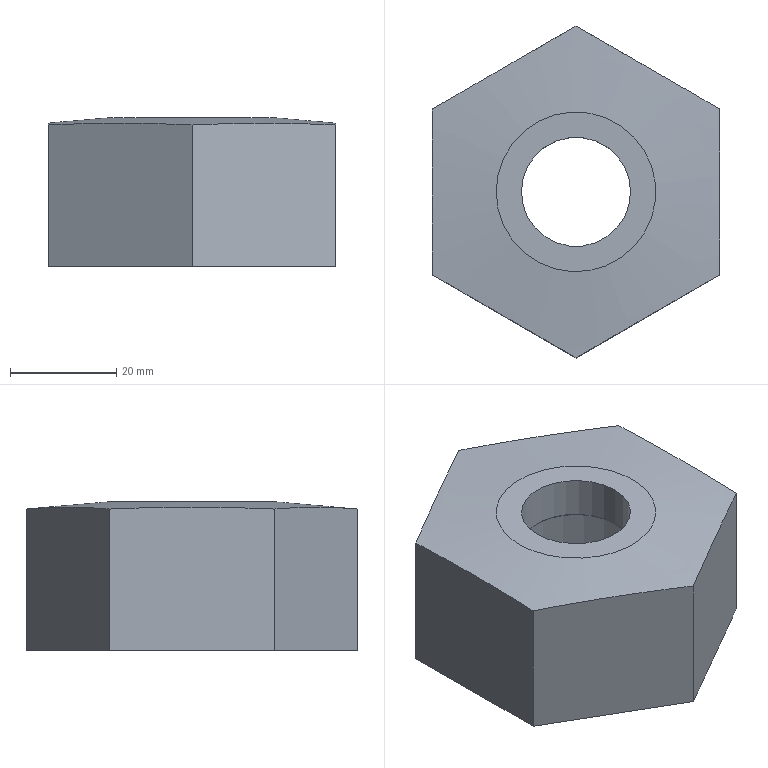Part | NX | features DATUM_CSYS 3, CYLINDER 2, SKETCH 2, CHAMFER 1, EXTRUDE 1, HOLE PACKAGE 1, SIMPLE HOLE 1, SWP104 1, SYMBOLIC_THREAD 1 | 1 solid | 16 faces | box 54.002 x 62.354 x 28 mm | volume 36749 mm3 | plane 10 | cylinder 3 | cone 3 | commonest cylinder face diameters 20.5 x1 43.5 x1 46 x1
STEP:
#1=CARTESIAN_POINT('',(10.25,0.,28.));
#2=VERTEX_POINT('',#1);
#3=CARTESIAN_POINT('',(0.,0.,28.));
#4=DIRECTION('',(0.,0.,1.));
#5=DIRECTION('',(1.,0.,0.));
#6=AXIS2_PLACEMENT_3D('',#3,#4,#5);
#7=CIRCLE('',#6,10.25);
#8=EDGE_CURVE('',#2,#2,#7,.T.);
#9=ORIENTED_EDGE('',*,*,#8,.F.);
#10=EDGE_LOOP('',(#9));
#11=FACE_BOUND('',#10,.T.);
#12=CARTESIAN_POINT('',(-15.,0.,28.));
#13=VERTEX_POINT('',#12);
#14=CARTESIAN_POINT('',(0.,0.,28.));
#15=DIRECTION('',(0.,0.,-1.));
#16=DIRECTION('',(-1.,0.,0.));
#17=AXIS2_PLACEMENT_3D('',#14,#15,#16);
#18=CIRCLE('',#17,15.);
#19=EDGE_CURVE('',#13,#13,#18,.T.);
#20=ORIENTED_EDGE('',*,*,#19,.F.);
#21=EDGE_LOOP('',(#20));
#22=FACE_BOUND('',#21,.T.);
#23=CARTESIAN_POINT('',(0.,0.,28.));
#24=DIRECTION('',(0.,0.,1.));
#25=DIRECTION('',(1.,0.,0.));
#26=AXIS2_PLACEMENT_3D('',#23,#24,#25);
#27=PLANE('',#26);
#28=ADVANCED_FACE('',(#11,#22),#27,.T.);
#29=CARTESIAN_POINT('',(-27.,-15.588,26.585));
#30=VERTEX_POINT('',#29);
#31=CARTESIAN_POINT('',(-27.,-15.588,0.));
#32=VERTEX_POINT('',#31);
#33=CARTESIAN_POINT('',(-27.,-15.588,28.));
#34=DIRECTION('',(0.,0.,-1.));
#35=VECTOR('',#34,1000.);
#36=LINE('',#33,#35);
#37=EDGE_CURVE('',#30,#32,#36,.T.);
#38=ORIENTED_EDGE('',*,*,#37,.F.);
#39=CARTESIAN_POINT('',(-27.,15.588,26.585));
#40=VERTEX_POINT('',#39);
#41=CARTESIAN_POINT('',(-27.,-15.588,26.585));
#42=CARTESIAN_POINT('',(-27.,-5.198,27.039));
#43=CARTESIAN_POINT('',(-27.,5.2,27.039));
#44=CARTESIAN_POINT('',(-27.,15.588,26.585));
#45=B_SPLINE_CURVE_WITH_KNOTS('',3,(#41,#42,#43,#44),.UNSPECIFIED.,.F.,.F.,(4,4),(0.02557,0.05677),.UNSPECIFIED.);
#46=EDGE_CURVE('',#30,#40,#45,.T.);
#47=ORIENTED_EDGE('',*,*,#46,.T.);
#48=CARTESIAN_POINT('',(-27.,15.588,0.));
#49=VERTEX_POINT('',#48);
#50=CARTESIAN_POINT('',(-27.,15.588,28.));
#51=DIRECTION('',(0.,0.,-1.));
#52=VECTOR('',#51,1000.);
#53=LINE('',#50,#52);
#54=EDGE_CURVE('',#40,#49,#53,.T.);
#55=ORIENTED_EDGE('',*,*,#54,.T.);
#56=CARTESIAN_POINT('',(-27.,15.588,0.));
#57=DIRECTION('',(0.,-1.,0.));
#58=VECTOR('',#57,1000.);
#59=LINE('',#56,#58);
#60=EDGE_CURVE('',#49,#32,#59,.T.);
#61=ORIENTED_EDGE('',*,*,#60,.T.);
#62=EDGE_LOOP('',(#38,#47,#55,#61));
#63=FACE_BOUND('',#62,.T.);
#64=CARTESIAN_POINT('',(-27.,15.588,28.));
#65=DIRECTION('',(1.,0.,0.));
#66=DIRECTION('',(0.,0.,-1.));
#67=AXIS2_PLACEMENT_3D('',#64,#65,#66);
#68=PLANE('',#67);
#69=ADVANCED_FACE('',(#63),#68,.F.);
#70=CARTESIAN_POINT('',(0.,-31.177,26.585));
#71=VERTEX_POINT('',#70);
#72=CARTESIAN_POINT('',(0.,-31.177,0.));
#73=VERTEX_POINT('',#72);
#74=CARTESIAN_POINT('',(0.,-31.177,28.));
#75=DIRECTION('',(0.,0.,-1.));
#76=VECTOR('',#75,1000.);
#77=LINE('',#74,#76);
#78=EDGE_CURVE('',#71,#73,#77,.T.);
#79=ORIENTED_EDGE('',*,*,#78,.F.);
#80=CARTESIAN_POINT('',(0.,-31.177,26.585));
#81=CARTESIAN_POINT('',(-9.,-25.981,27.039));
#82=CARTESIAN_POINT('',(-18.,-20.785,27.039));
#83=CARTESIAN_POINT('',(-27.,-15.588,26.585));
#84=B_SPLINE_CURVE_WITH_KNOTS('',3,(#80,#81,#82,#83),.UNSPECIFIED.,.F.,.F.,(4,4),(0.000000231,0.03118),.UNSPECIFIED.);
#85=EDGE_CURVE('',#71,#30,#84,.T.);
#86=ORIENTED_EDGE('',*,*,#85,.T.);
#87=ORIENTED_EDGE('',*,*,#37,.T.);
#88=CARTESIAN_POINT('',(-27.,-15.588,0.));
#89=DIRECTION('',(0.866,-0.5,0.));
#90=VECTOR('',#89,1000.);
#91=LINE('',#88,#90);
#92=EDGE_CURVE('',#32,#73,#91,.T.);
#93=ORIENTED_EDGE('',*,*,#92,.T.);
#94=EDGE_LOOP('',(#79,#86,#87,#93));
#95=FACE_BOUND('',#94,.T.);
#96=CARTESIAN_POINT('',(-27.,-15.588,28.));
#97=DIRECTION('',(0.5,0.866,0.));
#98=DIRECTION('',(-0.866,0.5,0.));
#99=AXIS2_PLACEMENT_3D('',#96,#97,#98);
#100=PLANE('',#99);
#101=ADVANCED_FACE('',(#95),#100,.F.);
#102=CARTESIAN_POINT('',(27.,-15.588,26.585));
#103=VERTEX_POINT('',#102);
#104=CARTESIAN_POINT('',(27.,-15.588,0.));
#105=VERTEX_POINT('',#104);
#106=CARTESIAN_POINT('',(27.,-15.588,28.));
#107=DIRECTION('',(0.,0.,-1.));
#108=VECTOR('',#107,1000.);
#109=LINE('',#106,#108);
#110=EDGE_CURVE('',#103,#105,#109,.T.);
#111=ORIENTED_EDGE('',*,*,#110,.F.);
#112=CARTESIAN_POINT('',(27.,-15.588,26.585));
#113=CARTESIAN_POINT('',(18.,-20.785,27.039));
#114=CARTESIAN_POINT('',(9.,-25.981,27.039));
#115=CARTESIAN_POINT('',(0.,-31.177,26.585));
#116=B_SPLINE_CURVE_WITH_KNOTS('',3,(#112,#113,#114,#115),.UNSPECIFIED.,.F.,.F.,(4,4),(0.000000231,0.03118),.UNSPECIFIED.);
#117=EDGE_CURVE('',#103,#71,#116,.T.);
#118=ORIENTED_EDGE('',*,*,#117,.T.);
#119=ORIENTED_EDGE('',*,*,#78,.T.);
#120=CARTESIAN_POINT('',(0.,-31.177,0.));
#121=DIRECTION('',(0.866,0.5,0.));
#122=VECTOR('',#121,1000.);
#123=LINE('',#120,#122);
#124=EDGE_CURVE('',#73,#105,#123,.T.);
#125=ORIENTED_EDGE('',*,*,#124,.T.);
#126=EDGE_LOOP('',(#111,#118,#119,#125));
#127=FACE_BOUND('',#126,.T.);
#128=CARTESIAN_POINT('',(0.,-31.177,28.));
#129=DIRECTION('',(-0.5,0.866,0.));
#130=DIRECTION('',(-0.866,-0.5,0.));
#131=AXIS2_PLACEMENT_3D('',#128,#129,#130);
#132=PLANE('',#131);
#133=ADVANCED_FACE('',(#127),#132,.F.);
#134=CARTESIAN_POINT('',(27.,15.588,26.585));
#135=VERTEX_POINT('',#134);
#136=CARTESIAN_POINT('',(27.,15.588,0.));
#137=VERTEX_POINT('',#136);
#138=CARTESIAN_POINT('',(27.,15.588,28.));
#139=DIRECTION('',(0.,0.,-1.));
#140=VECTOR('',#139,1000.);
#141=LINE('',#138,#140);
#142=EDGE_CURVE('',#135,#137,#141,.T.);
#143=ORIENTED_EDGE('',*,*,#142,.F.);
#144=CARTESIAN_POINT('',(27.,-15.588,26.585));
#145=CARTESIAN_POINT('',(27.,-5.198,27.039));
#146=CARTESIAN_POINT('',(27.,5.2,27.039));
#147=CARTESIAN_POINT('',(27.,15.588,26.585));
#148=B_SPLINE_CURVE_WITH_KNOTS('',3,(#144,#145,#146,#147),.UNSPECIFIED.,.F.,.F.,(4,4),(0.02557,0.05677),.UNSPECIFIED.);
#149=EDGE_CURVE('',#135,#103,#148,.F.);
#150=ORIENTED_EDGE('',*,*,#149,.T.);
#151=ORIENTED_EDGE('',*,*,#110,.T.);
#152=CARTESIAN_POINT('',(27.,-15.588,0.));
#153=DIRECTION('',(0.,1.,0.));
#154=VECTOR('',#153,1000.);
#155=LINE('',#152,#154);
#156=EDGE_CURVE('',#105,#137,#155,.T.);
#157=ORIENTED_EDGE('',*,*,#156,.T.);
#158=EDGE_LOOP('',(#143,#150,#151,#157));
#159=FACE_BOUND('',#158,.T.);
#160=CARTESIAN_POINT('',(27.,-15.588,28.));
#161=DIRECTION('',(-1.,0.,0.));
#162=DIRECTION('',(0.,-1.,0.));
#163=AXIS2_PLACEMENT_3D('',#160,#161,#162);
#164=PLANE('',#163);
#165=ADVANCED_FACE('',(#159),#164,.F.);
#166=CARTESIAN_POINT('',(0.,31.177,26.585));
#167=VERTEX_POINT('',#166);
#168=CARTESIAN_POINT('',(0.,31.177,0.));
#169=VERTEX_POINT('',#168);
#170=CARTESIAN_POINT('',(0.,31.177,28.));
#171=DIRECTION('',(0.,0.,-1.));
#172=VECTOR('',#171,1000.);
#173=LINE('',#170,#172);
#174=EDGE_CURVE('',#167,#169,#173,.T.);
#175=ORIENTED_EDGE('',*,*,#174,.F.);
#176=CARTESIAN_POINT('',(0.,31.177,26.585));
#177=CARTESIAN_POINT('',(9.,25.981,27.039));
#178=CARTESIAN_POINT('',(18.,20.785,27.039));
#179=CARTESIAN_POINT('',(27.,15.588,26.585));
#180=B_SPLINE_CURVE_WITH_KNOTS('',3,(#176,#177,#178,#179),.UNSPECIFIED.,.F.,.F.,(4,4),(0.000000231,0.03118),.UNSPECIFIED.);
#181=EDGE_CURVE('',#167,#135,#180,.T.);
#182=ORIENTED_EDGE('',*,*,#181,.T.);
#183=ORIENTED_EDGE('',*,*,#142,.T.);
#184=CARTESIAN_POINT('',(27.,15.588,0.));
#185=DIRECTION('',(-0.866,0.5,0.));
#186=VECTOR('',#185,1000.);
#187=LINE('',#184,#186);
#188=EDGE_CURVE('',#137,#169,#187,.T.);
#189=ORIENTED_EDGE('',*,*,#188,.T.);
#190=EDGE_LOOP('',(#175,#182,#183,#189));
#191=FACE_BOUND('',#190,.T.);
#192=CARTESIAN_POINT('',(27.,15.588,28.));
#193=DIRECTION('',(-0.5,-0.866,0.));
#194=DIRECTION('',(0.866,-0.5,0.));
#195=AXIS2_PLACEMENT_3D('',#192,#193,#194);
#196=PLANE('',#195);
#197=ADVANCED_FACE('',(#191),#196,.F.);
#198=ORIENTED_EDGE('',*,*,#54,.F.);
#199=CARTESIAN_POINT('',(-27.,15.588,26.585));
#200=CARTESIAN_POINT('',(-18.,20.785,27.039));
#201=CARTESIAN_POINT('',(-9.,25.981,27.039));
#202=CARTESIAN_POINT('',(0.,31.177,26.585));
#203=B_SPLINE_CURVE_WITH_KNOTS('',3,(#199,#200,#201,#202),.UNSPECIFIED.,.F.,.F.,(4,4),(0.000000231,0.03118),.UNSPECIFIED.);
#204=EDGE_CURVE('',#40,#167,#203,.T.);
#205=ORIENTED_EDGE('',*,*,#204,.T.);
#206=ORIENTED_EDGE('',*,*,#174,.T.);
#207=CARTESIAN_POINT('',(0.,31.177,0.));
#208=DIRECTION('',(-0.866,-0.5,0.));
#209=VECTOR('',#208,1000.);
#210=LINE('',#207,#209);
#211=EDGE_CURVE('',#169,#49,#210,.T.);
#212=ORIENTED_EDGE('',*,*,#211,.T.);
#213=EDGE_LOOP('',(#198,#205,#206,#212));
#214=FACE_BOUND('',#213,.T.);
#215=CARTESIAN_POINT('',(0.,31.177,28.));
#216=DIRECTION('',(0.5,-0.866,0.));
#217=DIRECTION('',(0.866,0.5,0.));
#218=AXIS2_PLACEMENT_3D('',#215,#216,#217);
#219=PLANE('',#218);
#220=ADVANCED_FACE('',(#214),#219,.F.);
#221=CARTESIAN_POINT('',(22.5,0.,0.));
#222=VERTEX_POINT('',#221);
#223=CARTESIAN_POINT('',(0.,0.,0.));
#224=DIRECTION('',(0.,0.,1.));
#225=DIRECTION('',(1.,0.,0.));
#226=AXIS2_PLACEMENT_3D('',#223,#224,#225);
#227=CIRCLE('',#226,22.5);
#228=EDGE_CURVE('',#222,#222,#227,.T.);
#229=ORIENTED_EDGE('',*,*,#228,.T.);
#230=EDGE_LOOP('',(#229));
#231=FACE_BOUND('',#230,.T.);
#232=ORIENTED_EDGE('',*,*,#60,.F.);
#233=ORIENTED_EDGE('',*,*,#211,.F.);
#234=ORIENTED_EDGE('',*,*,#188,.F.);
#235=ORIENTED_EDGE('',*,*,#156,.F.);
#236=ORIENTED_EDGE('',*,*,#124,.F.);
#237=ORIENTED_EDGE('',*,*,#92,.F.);
#238=EDGE_LOOP('',(#232,#233,#234,#235,#236,#237));
#239=FACE_BOUND('',#238,.T.);
#240=CARTESIAN_POINT('',(0.,0.,0.));
#241=DIRECTION('',(0.,0.,1.));
#242=DIRECTION('',(1.,0.,0.));
#243=AXIS2_PLACEMENT_3D('',#240,#241,#242);
#244=PLANE('',#243);
#245=ADVANCED_FACE('',(#231,#239),#244,.F.);
#246=CARTESIAN_POINT('',(21.75,0.,0.75));
#247=VERTEX_POINT('',#246);
#248=CARTESIAN_POINT('',(0.,0.,0.75));
#249=DIRECTION('',(0.,0.,1.));
#250=DIRECTION('',(1.,0.,0.));
#251=AXIS2_PLACEMENT_3D('',#248,#249,#250);
#252=CIRCLE('',#251,21.75);
#253=EDGE_CURVE('',#247,#247,#252,.F.);
#254=ORIENTED_EDGE('',*,*,#253,.T.);
#255=EDGE_LOOP('',(#254));
#256=FACE_BOUND('',#255,.T.);
#257=CARTESIAN_POINT('',(21.75,0.,18.));
#258=VERTEX_POINT('',#257);
#259=CARTESIAN_POINT('',(0.,0.,18.));
#260=DIRECTION('',(0.,0.,1.));
#261=DIRECTION('',(1.,0.,0.));
#262=AXIS2_PLACEMENT_3D('',#259,#260,#261);
#263=CIRCLE('',#262,21.75);
#264=EDGE_CURVE('',#258,#258,#263,.F.);
#265=ORIENTED_EDGE('',*,*,#264,.F.);
#266=EDGE_LOOP('',(#265));
#267=FACE_BOUND('',#266,.T.);
#268=CARTESIAN_POINT('',(0.,0.,0.));
#269=DIRECTION('',(0.,0.,1.));
#270=DIRECTION('',(1.,0.,0.));
#271=AXIS2_PLACEMENT_3D('',#268,#269,#270);
#272=CYLINDRICAL_SURFACE('',#271,21.75);
#273=ADVANCED_FACE('',(#256,#267),#272,.F.);
#274=ORIENTED_EDGE('',*,*,#253,.F.);
#275=EDGE_LOOP('',(#274));
#276=FACE_BOUND('',#275,.T.);
#277=ORIENTED_EDGE('',*,*,#228,.F.);
#278=EDGE_LOOP('',(#277));
#279=FACE_BOUND('',#278,.T.);
#280=CARTESIAN_POINT('',(0.,0.,0.));
#281=DIRECTION('',(0.,0.,-1.));
#282=DIRECTION('',(-1.,0.,0.));
#283=AXIS2_PLACEMENT_3D('',#280,#281,#282);
#284=CONICAL_SURFACE('',#283,22.5,0.7854);
#285=ADVANCED_FACE('',(#276,#279),#284,.F.);
#286=CARTESIAN_POINT('',(10.5,0.,20.));
#287=VERTEX_POINT('',#286);
#288=CARTESIAN_POINT('',(0.,0.,20.));
#289=DIRECTION('',(0.,0.,1.));
#290=DIRECTION('',(1.,0.,0.));
#291=AXIS2_PLACEMENT_3D('',#288,#289,#290);
#292=CIRCLE('',#291,10.5);
#293=EDGE_CURVE('',#287,#287,#292,.T.);
#294=ORIENTED_EDGE('',*,*,#293,.T.);
#295=EDGE_LOOP('',(#294));
#296=FACE_BOUND('',#295,.T.);
#297=CARTESIAN_POINT('',(23.,0.,20.));
#298=VERTEX_POINT('',#297);
#299=CARTESIAN_POINT('',(0.,0.,20.));
#300=DIRECTION('',(0.,0.,-1.));
#301=DIRECTION('',(1.,0.,0.));
#302=AXIS2_PLACEMENT_3D('',#299,#300,#301);
#303=CIRCLE('',#302,23.);
#304=EDGE_CURVE('',#298,#298,#303,.F.);
#305=ORIENTED_EDGE('',*,*,#304,.F.);
#306=EDGE_LOOP('',(#305));
#307=FACE_BOUND('',#306,.T.);
#308=CARTESIAN_POINT('',(0.,0.,20.));
#309=DIRECTION('',(0.,0.,1.));
#310=DIRECTION('',(1.,0.,0.));
#311=AXIS2_PLACEMENT_3D('',#308,#309,#310);
#312=PLANE('',#311);
#313=ADVANCED_FACE('',(#296,#307),#312,.F.);
#314=ORIENTED_EDGE('',*,*,#264,.T.);
#315=EDGE_LOOP('',(#314));
#316=FACE_BOUND('',#315,.T.);
#317=CARTESIAN_POINT('',(23.,0.,18.));
#318=VERTEX_POINT('',#317);
#319=CARTESIAN_POINT('',(0.,0.,18.));
#320=DIRECTION('',(0.,0.,1.));
#321=DIRECTION('',(1.,0.,0.));
#322=AXIS2_PLACEMENT_3D('',#319,#320,#321);
#323=CIRCLE('',#322,23.);
#324=EDGE_CURVE('',#318,#318,#323,.F.);
#325=ORIENTED_EDGE('',*,*,#324,.F.);
#326=EDGE_LOOP('',(#325));
#327=FACE_BOUND('',#326,.T.);
#328=CARTESIAN_POINT('',(0.,0.,18.));
#329=DIRECTION('',(0.,0.,-1.));
#330=DIRECTION('',(-1.,0.,0.));
#331=AXIS2_PLACEMENT_3D('',#328,#329,#330);
#332=PLANE('',#331);
#333=ADVANCED_FACE('',(#316,#327),#332,.F.);
#334=ORIENTED_EDGE('',*,*,#304,.T.);
#335=EDGE_LOOP('',(#334));
#336=FACE_BOUND('',#335,.T.);
#337=ORIENTED_EDGE('',*,*,#324,.T.);
#338=EDGE_LOOP('',(#337));
#339=FACE_BOUND('',#338,.T.);
#340=CARTESIAN_POINT('',(0.,0.,18.));
#341=DIRECTION('',(0.,0.,1.));
#342=DIRECTION('',(1.,0.,0.));
#343=AXIS2_PLACEMENT_3D('',#340,#341,#342);
#344=CYLINDRICAL_SURFACE('',#343,23.);
#345=ADVANCED_FACE('',(#336,#339),#344,.F.);
#346=CARTESIAN_POINT('',(10.25,0.,20.25));
#347=VERTEX_POINT('',#346);
#348=CARTESIAN_POINT('',(0.,0.,20.25));
#349=DIRECTION('',(0.,0.,1.));
#350=DIRECTION('',(1.,0.,0.));
#351=AXIS2_PLACEMENT_3D('',#348,#349,#350);
#352=CIRCLE('',#351,10.25);
#353=EDGE_CURVE('',#347,#347,#352,.F.);
#354=ORIENTED_EDGE('',*,*,#353,.T.);
#355=EDGE_LOOP('',(#354));
#356=FACE_BOUND('',#355,.T.);
#357=ORIENTED_EDGE('',*,*,#8,.T.);
#358=EDGE_LOOP('',(#357));
#359=FACE_BOUND('',#358,.T.);
#360=CARTESIAN_POINT('',(0.,0.,20.));
#361=DIRECTION('',(0.,0.,1.));
#362=DIRECTION('',(1.,0.,0.));
#363=AXIS2_PLACEMENT_3D('',#360,#361,#362);
#364=CYLINDRICAL_SURFACE('',#363,10.25);
#365=ADVANCED_FACE('',(#356,#359),#364,.F.);
#366=ORIENTED_EDGE('',*,*,#19,.T.);
#367=EDGE_LOOP('',(#366));
#368=FACE_BOUND('',#367,.T.);
#369=ORIENTED_EDGE('',*,*,#85,.F.);
#370=ORIENTED_EDGE('',*,*,#117,.F.);
#371=ORIENTED_EDGE('',*,*,#149,.F.);
#372=ORIENTED_EDGE('',*,*,#181,.F.);
#373=ORIENTED_EDGE('',*,*,#204,.F.);
#374=ORIENTED_EDGE('',*,*,#46,.F.);
#375=EDGE_LOOP('',(#369,#370,#371,#372,#373,#374));
#376=FACE_BOUND('',#375,.T.);
#377=CARTESIAN_POINT('',(0.,0.,28.));
#378=DIRECTION('',(0.,0.,-1.));
#379=DIRECTION('',(-1.,0.,0.));
#380=AXIS2_PLACEMENT_3D('',#377,#378,#379);
#381=CONICAL_SURFACE('',#380,15.,1.484);
#382=ADVANCED_FACE('',(#368,#376),#381,.T.);
#383=ORIENTED_EDGE('',*,*,#353,.F.);
#384=EDGE_LOOP('',(#383));
#385=FACE_BOUND('',#384,.T.);
#386=ORIENTED_EDGE('',*,*,#293,.F.);
#387=EDGE_LOOP('',(#386));
#388=FACE_BOUND('',#387,.T.);
#389=CARTESIAN_POINT('',(0.,0.,20.));
#390=DIRECTION('',(0.,0.,-1.));
#391=DIRECTION('',(-1.,0.,0.));
#392=AXIS2_PLACEMENT_3D('',#389,#390,#391);
#393=CONICAL_SURFACE('',#392,10.5,0.7854);
#394=ADVANCED_FACE('',(#385,#388),#393,.F.);
#395=CLOSED_SHELL('',(#28,#69,#101,#133,#165,#197,#220,#245,#273,#285,#313,#333,#345,#365,#382,#394));
#396=MANIFOLD_SOLID_BREP('',#395);
#397=(LENGTH_UNIT()NAMED_UNIT(*)SI_UNIT(.MILLI.,.METRE.));
#398=UNCERTAINTY_MEASURE_WITH_UNIT(LENGTH_MEASURE(0.0508),#397,'','');
#399=(NAMED_UNIT(*)PLANE_ANGLE_UNIT()SI_UNIT($,.RADIAN.));
#400=(NAMED_UNIT(*)SI_UNIT($,.STERADIAN.)SOLID_ANGLE_UNIT());
#401=(GEOMETRIC_REPRESENTATION_CONTEXT(3)GLOBAL_UNCERTAINTY_ASSIGNED_CONTEXT((#398))GLOBAL_UNIT_ASSIGNED_CONTEXT((#397,#399,#400))REPRESENTATION_CONTEXT('',''));
#402=ADVANCED_BREP_SHAPE_REPRESENTATION('',(#396),#401);